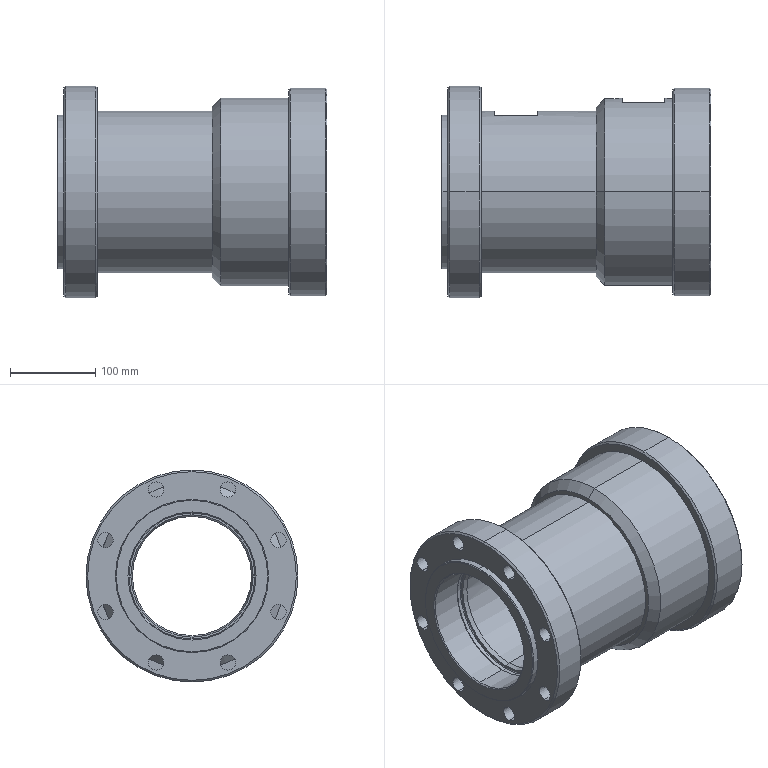Part | SolidWorks | features Chamfer 8, HoleWzd 6, ICE 5, Cut 1, Fillet 1, LibraryFeature 1, Revolution 1 | 1 solid | 198 faces | box 317 x 249 x 249 mm | volume 6036986 mm3 | cylinder 104 | cone 64 | plane 26 | torus 4 | commonest cylinder face diameters 14 x24 16 x24 5 x16 18 x16 15 x4 140 x2